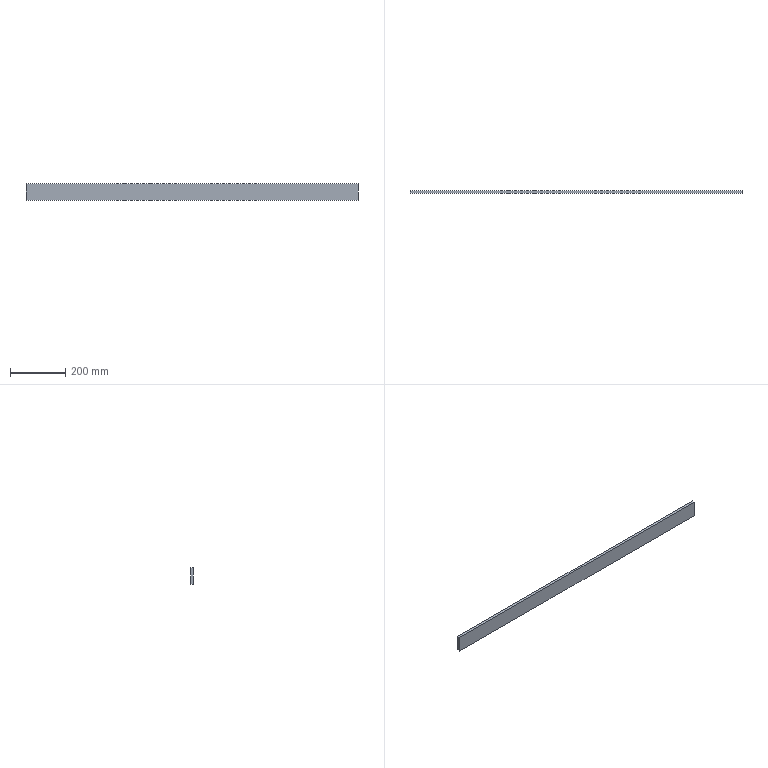Part | SolidWorks | features FlatPattern 1, SMBaseFlange 1, SheetMetal 1 | 1 solid | 6 faces | box 1200 x 10 x 60 mm | volume 720000 mm3 | plane 6
STEP:
#1=CARTESIAN_POINT('',(600.,0.,30.));
#2=VERTEX_POINT('',#1);
#3=CARTESIAN_POINT('',(600.,0.,-30.));
#4=VERTEX_POINT('',#3);
#5=CARTESIAN_POINT('',(600.,0.,-30.));
#6=DIRECTION('',(0.,0.,-1.));
#7=VECTOR('',#6,1000.);
#8=LINE('',#5,#7);
#9=EDGE_CURVE('',#2,#4,#8,.T.);
#10=ORIENTED_EDGE('',*,*,#9,.F.);
#11=CARTESIAN_POINT('',(600.,-10.,30.));
#12=VERTEX_POINT('',#11);
#13=CARTESIAN_POINT('',(600.,-10.,30.));
#14=DIRECTION('',(0.,1.,0.));
#15=VECTOR('',#14,1000.);
#16=LINE('',#13,#15);
#17=EDGE_CURVE('',#12,#2,#16,.T.);
#18=ORIENTED_EDGE('',*,*,#17,.F.);
#19=CARTESIAN_POINT('',(600.,-10.,-30.));
#20=VERTEX_POINT('',#19);
#21=CARTESIAN_POINT('',(600.,-10.,-30.));
#22=DIRECTION('',(0.,0.,-1.));
#23=VECTOR('',#22,1000.);
#24=LINE('',#21,#23);
#25=EDGE_CURVE('',#12,#20,#24,.T.);
#26=ORIENTED_EDGE('',*,*,#25,.T.);
#27=CARTESIAN_POINT('',(600.,-10.,-30.));
#28=DIRECTION('',(0.,1.,0.));
#29=VECTOR('',#28,1000.);
#30=LINE('',#27,#29);
#31=EDGE_CURVE('',#20,#4,#30,.T.);
#32=ORIENTED_EDGE('',*,*,#31,.T.);
#33=EDGE_LOOP('',(#10,#18,#26,#32));
#34=FACE_OUTER_BOUND('',#33,.T.);
#35=CARTESIAN_POINT('',(600.,-10.,-30.));
#36=DIRECTION('',(1.,0.,0.));
#37=DIRECTION('',(0.,0.,-1.));
#38=AXIS2_PLACEMENT_3D('',#35,#36,#37);
#39=PLANE('',#38);
#40=ADVANCED_FACE('',(#34),#39,.T.);
#41=CARTESIAN_POINT('',(-600.,0.,30.));
#42=VERTEX_POINT('',#41);
#43=CARTESIAN_POINT('',(-600.,0.,30.));
#44=DIRECTION('',(1.,0.,0.));
#45=VECTOR('',#44,1000.);
#46=LINE('',#43,#45);
#47=EDGE_CURVE('',#42,#2,#46,.T.);
#48=ORIENTED_EDGE('',*,*,#47,.F.);
#49=CARTESIAN_POINT('',(-600.,-10.,30.));
#50=VERTEX_POINT('',#49);
#51=CARTESIAN_POINT('',(-600.,-10.,30.));
#52=DIRECTION('',(0.,1.,0.));
#53=VECTOR('',#52,1000.);
#54=LINE('',#51,#53);
#55=EDGE_CURVE('',#50,#42,#54,.T.);
#56=ORIENTED_EDGE('',*,*,#55,.F.);
#57=CARTESIAN_POINT('',(-600.,-10.,30.));
#58=DIRECTION('',(1.,0.,0.));
#59=VECTOR('',#58,1000.);
#60=LINE('',#57,#59);
#61=EDGE_CURVE('',#50,#12,#60,.T.);
#62=ORIENTED_EDGE('',*,*,#61,.T.);
#63=ORIENTED_EDGE('',*,*,#17,.T.);
#64=EDGE_LOOP('',(#48,#56,#62,#63));
#65=FACE_OUTER_BOUND('',#64,.T.);
#66=CARTESIAN_POINT('',(-600.,-10.,30.));
#67=DIRECTION('',(0.,0.,1.));
#68=DIRECTION('',(1.,0.,0.));
#69=AXIS2_PLACEMENT_3D('',#66,#67,#68);
#70=PLANE('',#69);
#71=ADVANCED_FACE('',(#65),#70,.T.);
#72=CARTESIAN_POINT('',(-600.,0.,-30.));
#73=VERTEX_POINT('',#72);
#74=CARTESIAN_POINT('',(-600.,0.,-30.));
#75=DIRECTION('',(0.,0.,1.));
#76=VECTOR('',#75,1000.);
#77=LINE('',#74,#76);
#78=EDGE_CURVE('',#73,#42,#77,.T.);
#79=ORIENTED_EDGE('',*,*,#78,.F.);
#80=CARTESIAN_POINT('',(-600.,-10.,-30.));
#81=VERTEX_POINT('',#80);
#82=CARTESIAN_POINT('',(-600.,-10.,-30.));
#83=DIRECTION('',(0.,1.,0.));
#84=VECTOR('',#83,1000.);
#85=LINE('',#82,#84);
#86=EDGE_CURVE('',#81,#73,#85,.T.);
#87=ORIENTED_EDGE('',*,*,#86,.F.);
#88=CARTESIAN_POINT('',(-600.,-10.,-30.));
#89=DIRECTION('',(0.,0.,1.));
#90=VECTOR('',#89,1000.);
#91=LINE('',#88,#90);
#92=EDGE_CURVE('',#81,#50,#91,.T.);
#93=ORIENTED_EDGE('',*,*,#92,.T.);
#94=ORIENTED_EDGE('',*,*,#55,.T.);
#95=EDGE_LOOP('',(#79,#87,#93,#94));
#96=FACE_OUTER_BOUND('',#95,.T.);
#97=CARTESIAN_POINT('',(-600.,-10.,-30.));
#98=DIRECTION('',(-1.,0.,0.));
#99=DIRECTION('',(0.,0.,1.));
#100=AXIS2_PLACEMENT_3D('',#97,#98,#99);
#101=PLANE('',#100);
#102=ADVANCED_FACE('',(#96),#101,.T.);
#103=CARTESIAN_POINT('',(-600.,0.,-30.));
#104=DIRECTION('',(-1.,0.,0.));
#105=VECTOR('',#104,1000.);
#106=LINE('',#103,#105);
#107=EDGE_CURVE('',#4,#73,#106,.T.);
#108=ORIENTED_EDGE('',*,*,#107,.F.);
#109=ORIENTED_EDGE('',*,*,#31,.F.);
#110=CARTESIAN_POINT('',(-600.,-10.,-30.));
#111=DIRECTION('',(-1.,0.,0.));
#112=VECTOR('',#111,1000.);
#113=LINE('',#110,#112);
#114=EDGE_CURVE('',#20,#81,#113,.T.);
#115=ORIENTED_EDGE('',*,*,#114,.T.);
#116=ORIENTED_EDGE('',*,*,#86,.T.);
#117=EDGE_LOOP('',(#108,#109,#115,#116));
#118=FACE_OUTER_BOUND('',#117,.T.);
#119=CARTESIAN_POINT('',(-600.,-10.,-30.));
#120=DIRECTION('',(0.,0.,-1.));
#121=DIRECTION('',(-1.,0.,0.));
#122=AXIS2_PLACEMENT_3D('',#119,#120,#121);
#123=PLANE('',#122);
#124=ADVANCED_FACE('',(#118),#123,.T.);
#125=ORIENTED_EDGE('',*,*,#25,.F.);
#126=ORIENTED_EDGE('',*,*,#61,.F.);
#127=ORIENTED_EDGE('',*,*,#92,.F.);
#128=ORIENTED_EDGE('',*,*,#114,.F.);
#129=EDGE_LOOP('',(#125,#126,#127,#128));
#130=FACE_OUTER_BOUND('',#129,.T.);
#131=CARTESIAN_POINT('',(0.,-10.,0.));
#132=DIRECTION('',(0.,1.,0.));
#133=DIRECTION('',(0.,0.,1.));
#134=AXIS2_PLACEMENT_3D('',#131,#132,#133);
#135=PLANE('',#134);
#136=ADVANCED_FACE('',(#130),#135,.F.);
#137=ORIENTED_EDGE('',*,*,#9,.T.);
#138=ORIENTED_EDGE('',*,*,#107,.T.);
#139=ORIENTED_EDGE('',*,*,#78,.T.);
#140=ORIENTED_EDGE('',*,*,#47,.T.);
#141=EDGE_LOOP('',(#137,#138,#139,#140));
#142=FACE_OUTER_BOUND('',#141,.T.);
#143=CARTESIAN_POINT('',(0.,0.,0.));
#144=DIRECTION('',(0.,1.,0.));
#145=DIRECTION('',(0.,0.,1.));
#146=AXIS2_PLACEMENT_3D('',#143,#144,#145);
#147=PLANE('',#146);
#148=ADVANCED_FACE('',(#142),#147,.T.);
#149=CLOSED_SHELL('',(#40,#71,#102,#124,#136,#148));
#150=MANIFOLD_SOLID_BREP('',#149);
#151=CARTESIAN_POINT('',(0.,0.,0.));
#152=DIRECTION('',(0.,0.,1.));
#153=DIRECTION('',(1.,0.,0.));
#154=AXIS2_PLACEMENT_3D('',#151,#152,#153);
#155=(LENGTH_UNIT()NAMED_UNIT(*)SI_UNIT(.MILLI.,.METRE.));
#156=UNCERTAINTY_MEASURE_WITH_UNIT(LENGTH_MEASURE(0.00001),#155,'','');
#157=(NAMED_UNIT(*)PLANE_ANGLE_UNIT()SI_UNIT($,.RADIAN.));
#158=(NAMED_UNIT(*)SI_UNIT($,.STERADIAN.)SOLID_ANGLE_UNIT());
#159=(GEOMETRIC_REPRESENTATION_CONTEXT(3)GLOBAL_UNCERTAINTY_ASSIGNED_CONTEXT((#156))GLOBAL_UNIT_ASSIGNED_CONTEXT((#155,#157,#158))REPRESENTATION_CONTEXT('',''));
#160=ADVANCED_BREP_SHAPE_REPRESENTATION('',(#150,#154),#159);